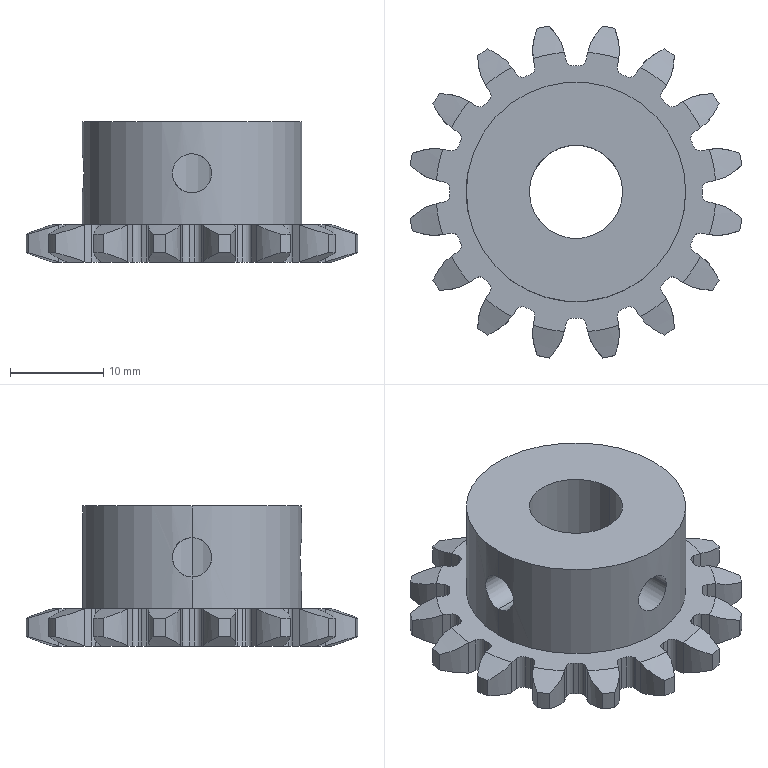Part | STEP file | Sprocket 1/4in-10 | 1 solid | 180 faces | box 35.544 x 35.544 x 15 mm | volume 6436 mm3 | cylinder 81 | plane 35 | cone 32 | spline 32 | commonest cylinder face diameters 1.52 x40 27 x17 36 x16 4.2 x4 10 x2 23.5 x2